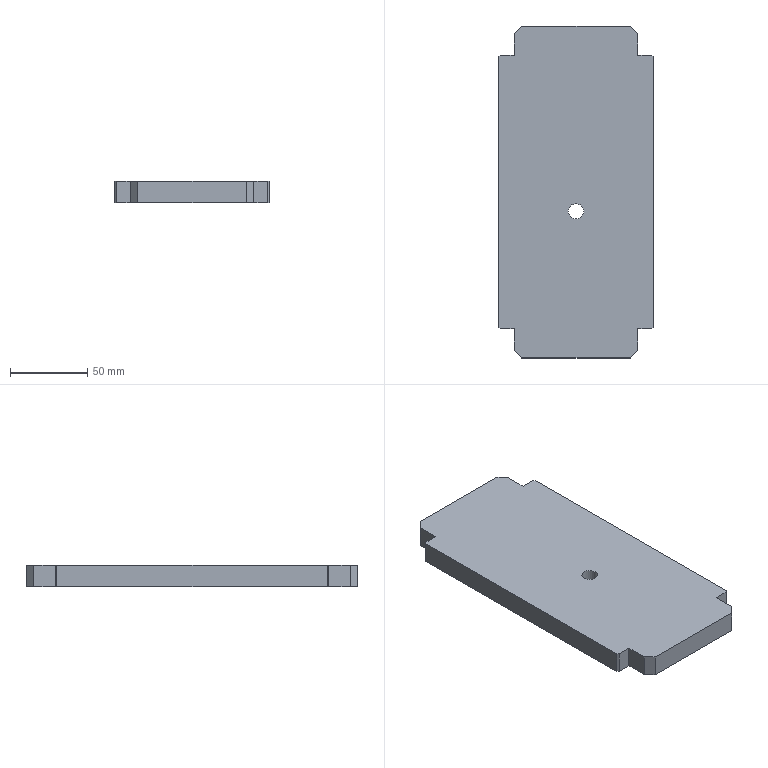Part | NX | features solid 2 | 1 solid | 23 faces | box 100 x 215 x 14 mm | volume 288532 mm3 | plane 22 | cylinder 1 | commonest cylinder face diameters 10 x1
STEP:
#1=CARTESIAN_POINT('',(-25.,296.,-5.));
#2=VERTEX_POINT('',#1);
#3=CARTESIAN_POINT('',(-34.,296.,-5.));
#4=VERTEX_POINT('',#3);
#5=CARTESIAN_POINT('',(300.,296.,-5.));
#6=DIRECTION('',(-1.,0.,0.));
#7=VECTOR('',#6,1000.);
#8=LINE('',#5,#7);
#9=EDGE_CURVE('',#2,#4,#8,.T.);
#10=ORIENTED_EDGE('',*,*,#9,.F.);
#11=CARTESIAN_POINT('',(-25.,296.,-19.));
#12=VERTEX_POINT('',#11);
#13=CARTESIAN_POINT('',(-25.,296.,-21.));
#14=DIRECTION('',(0.,0.,-1.));
#15=VECTOR('',#14,1000.);
#16=LINE('',#13,#15);
#17=EDGE_CURVE('',#2,#12,#16,.T.);
#18=ORIENTED_EDGE('',*,*,#17,.T.);
#19=CARTESIAN_POINT('',(-34.,296.,-19.));
#20=VERTEX_POINT('',#19);
#21=CARTESIAN_POINT('',(15.,296.,-19.));
#22=DIRECTION('',(-1.,0.,0.));
#23=VECTOR('',#22,1000.);
#24=LINE('',#21,#23);
#25=EDGE_CURVE('',#12,#20,#24,.T.);
#26=ORIENTED_EDGE('',*,*,#25,.T.);
#27=CARTESIAN_POINT('',(-34.,296.,-21.));
#28=DIRECTION('',(0.,0.,1.));
#29=VECTOR('',#28,1000.);
#30=LINE('',#27,#29);
#31=EDGE_CURVE('',#20,#4,#30,.T.);
#32=ORIENTED_EDGE('',*,*,#31,.T.);
#33=EDGE_LOOP('',(#10,#18,#26,#32));
#34=FACE_BOUND('',#33,.T.);
#35=CARTESIAN_POINT('',(300.,296.,-21.));
#36=DIRECTION('',(0.,1.,0.));
#37=DIRECTION('',(0.,0.,1.));
#38=AXIS2_PLACEMENT_3D('',#35,#36,#37);
#39=PLANE('',#38);
#40=ADVANCED_FACE('',(#34),#39,.T.);
#41=CARTESIAN_POINT('',(-34.,119.,-19.));
#42=VERTEX_POINT('',#41);
#43=CARTESIAN_POINT('',(-25.,119.,-19.));
#44=VERTEX_POINT('',#43);
#45=CARTESIAN_POINT('',(15.,119.,-19.));
#46=DIRECTION('',(1.,0.,0.));
#47=VECTOR('',#46,1000.);
#48=LINE('',#45,#47);
#49=EDGE_CURVE('',#42,#44,#48,.T.);
#50=ORIENTED_EDGE('',*,*,#49,.T.);
#51=CARTESIAN_POINT('',(-25.,119.,-5.));
#52=VERTEX_POINT('',#51);
#53=CARTESIAN_POINT('',(-25.,119.,-21.));
#54=DIRECTION('',(0.,0.,1.));
#55=VECTOR('',#54,1000.);
#56=LINE('',#53,#55);
#57=EDGE_CURVE('',#44,#52,#56,.T.);
#58=ORIENTED_EDGE('',*,*,#57,.T.);
#59=CARTESIAN_POINT('',(-34.,119.,-5.));
#60=VERTEX_POINT('',#59);
#61=CARTESIAN_POINT('',(-285.,119.,-5.));
#62=DIRECTION('',(1.,0.,0.));
#63=VECTOR('',#62,1000.);
#64=LINE('',#61,#63);
#65=EDGE_CURVE('',#60,#52,#64,.T.);
#66=ORIENTED_EDGE('',*,*,#65,.F.);
#67=CARTESIAN_POINT('',(-34.,119.,-21.));
#68=DIRECTION('',(0.,0.,1.));
#69=VECTOR('',#68,1000.);
#70=LINE('',#67,#69);
#71=EDGE_CURVE('',#42,#60,#70,.T.);
#72=ORIENTED_EDGE('',*,*,#71,.F.);
#73=EDGE_LOOP('',(#50,#58,#66,#72));
#74=FACE_BOUND('',#73,.T.);
#75=CARTESIAN_POINT('',(-285.,119.,-21.));
#76=DIRECTION('',(0.,-1.,0.));
#77=DIRECTION('',(1.,0.,0.));
#78=AXIS2_PLACEMENT_3D('',#75,#76,#77);
#79=PLANE('',#78);
#80=ADVANCED_FACE('',(#74),#79,.T.);
#81=CARTESIAN_POINT('',(55.,296.,-5.));
#82=VERTEX_POINT('',#81);
#83=CARTESIAN_POINT('',(55.,296.,-19.));
#84=VERTEX_POINT('',#83);
#85=CARTESIAN_POINT('',(55.,296.,-21.));
#86=DIRECTION('',(0.,0.,-1.));
#87=VECTOR('',#86,1000.);
#88=LINE('',#85,#87);
#89=EDGE_CURVE('',#82,#84,#88,.T.);
#90=ORIENTED_EDGE('',*,*,#89,.F.);
#91=CARTESIAN_POINT('',(64.,296.,-5.));
#92=VERTEX_POINT('',#91);
#93=CARTESIAN_POINT('',(300.,296.,-5.));
#94=DIRECTION('',(-1.,0.,0.));
#95=VECTOR('',#94,1000.);
#96=LINE('',#93,#95);
#97=EDGE_CURVE('',#92,#82,#96,.T.);
#98=ORIENTED_EDGE('',*,*,#97,.F.);
#99=CARTESIAN_POINT('',(64.,296.,-19.));
#100=VERTEX_POINT('',#99);
#101=CARTESIAN_POINT('',(64.,296.,-21.));
#102=DIRECTION('',(0.,0.,1.));
#103=VECTOR('',#102,1000.);
#104=LINE('',#101,#103);
#105=EDGE_CURVE('',#100,#92,#104,.T.);
#106=ORIENTED_EDGE('',*,*,#105,.F.);
#107=CARTESIAN_POINT('',(15.,296.,-19.));
#108=DIRECTION('',(-1.,0.,0.));
#109=VECTOR('',#108,1000.);
#110=LINE('',#107,#109);
#111=EDGE_CURVE('',#100,#84,#110,.T.);
#112=ORIENTED_EDGE('',*,*,#111,.T.);
#113=EDGE_LOOP('',(#90,#98,#106,#112));
#114=FACE_BOUND('',#113,.T.);
#115=CARTESIAN_POINT('',(300.,296.,-21.));
#116=DIRECTION('',(0.,1.,0.));
#117=DIRECTION('',(0.,0.,1.));
#118=AXIS2_PLACEMENT_3D('',#115,#116,#117);
#119=PLANE('',#118);
#120=ADVANCED_FACE('',(#114),#119,.T.);
#121=CARTESIAN_POINT('',(-35.,295.,-5.));
#122=VERTEX_POINT('',#121);
#123=CARTESIAN_POINT('',(-34.,296.,-5.));
#124=DIRECTION('',(-0.7071,-0.7071,0.));
#125=VECTOR('',#124,1000.);
#126=LINE('',#123,#125);
#127=EDGE_CURVE('',#4,#122,#126,.T.);
#128=ORIENTED_EDGE('',*,*,#127,.F.);
#129=ORIENTED_EDGE('',*,*,#31,.F.);
#130=CARTESIAN_POINT('',(-35.,295.,-19.));
#131=VERTEX_POINT('',#130);
#132=CARTESIAN_POINT('',(-60.,270.,-19.));
#133=DIRECTION('',(-0.7071,-0.7071,0.));
#134=VECTOR('',#133,1000.);
#135=LINE('',#132,#134);
#136=EDGE_CURVE('',#20,#131,#135,.T.);
#137=ORIENTED_EDGE('',*,*,#136,.T.);
#138=CARTESIAN_POINT('',(-35.,295.,-21.));
#139=DIRECTION('',(0.,0.,1.));
#140=VECTOR('',#139,1000.);
#141=LINE('',#138,#140);
#142=EDGE_CURVE('',#131,#122,#141,.T.);
#143=ORIENTED_EDGE('',*,*,#142,.T.);
#144=EDGE_LOOP('',(#128,#129,#137,#143));
#145=FACE_BOUND('',#144,.T.);
#146=CARTESIAN_POINT('',(-34.,296.,-21.));
#147=DIRECTION('',(-0.7071,0.7071,0.));
#148=DIRECTION('',(-0.7071,-0.7071,0.));
#149=AXIS2_PLACEMENT_3D('',#146,#147,#148);
#150=PLANE('',#149);
#151=ADVANCED_FACE('',(#145),#150,.T.);
#152=CARTESIAN_POINT('',(-35.,120.,-5.));
#153=VERTEX_POINT('',#152);
#154=CARTESIAN_POINT('',(-35.,195.,-5.));
#155=DIRECTION('',(0.,1.,0.));
#156=VECTOR('',#155,1000.);
#157=LINE('',#154,#156);
#158=EDGE_CURVE('',#153,#122,#157,.T.);
#159=ORIENTED_EDGE('',*,*,#158,.T.);
#160=ORIENTED_EDGE('',*,*,#142,.F.);
#161=CARTESIAN_POINT('',(-35.,120.,-19.));
#162=VERTEX_POINT('',#161);
#163=CARTESIAN_POINT('',(-35.,195.,-19.));
#164=DIRECTION('',(0.,1.,0.));
#165=VECTOR('',#164,1000.);
#166=LINE('',#163,#165);
#167=EDGE_CURVE('',#162,#131,#166,.T.);
#168=ORIENTED_EDGE('',*,*,#167,.F.);
#169=CARTESIAN_POINT('',(-35.,120.,-21.));
#170=DIRECTION('',(0.,0.,1.));
#171=VECTOR('',#170,1000.);
#172=LINE('',#169,#171);
#173=EDGE_CURVE('',#162,#153,#172,.T.);
#174=ORIENTED_EDGE('',*,*,#173,.T.);
#175=EDGE_LOOP('',(#159,#160,#168,#174));
#176=FACE_BOUND('',#175,.T.);
#177=CARTESIAN_POINT('',(-35.,195.,-21.));
#178=DIRECTION('',(1.,0.,0.));
#179=DIRECTION('',(0.,1.,0.));
#180=AXIS2_PLACEMENT_3D('',#177,#178,#179);
#181=PLANE('',#180);
#182=ADVANCED_FACE('',(#176),#181,.F.);
#183=CARTESIAN_POINT('',(-35.,120.,-5.));
#184=DIRECTION('',(0.7071,-0.7071,0.));
#185=VECTOR('',#184,1000.);
#186=LINE('',#183,#185);
#187=EDGE_CURVE('',#153,#60,#186,.T.);
#188=ORIENTED_EDGE('',*,*,#187,.F.);
#189=ORIENTED_EDGE('',*,*,#173,.F.);
#190=CARTESIAN_POINT('',(-47.5,132.5,-19.));
#191=DIRECTION('',(0.7071,-0.7071,0.));
#192=VECTOR('',#191,1000.);
#193=LINE('',#190,#192);
#194=EDGE_CURVE('',#162,#42,#193,.T.);
#195=ORIENTED_EDGE('',*,*,#194,.T.);
#196=ORIENTED_EDGE('',*,*,#71,.T.);
#197=EDGE_LOOP('',(#188,#189,#195,#196));
#198=FACE_BOUND('',#197,.T.);
#199=CARTESIAN_POINT('',(-35.,120.,-21.));
#200=DIRECTION('',(-0.7071,-0.7071,0.));
#201=DIRECTION('',(0.7071,-0.7071,0.));
#202=AXIS2_PLACEMENT_3D('',#199,#200,#201);
#203=PLANE('',#202);
#204=ADVANCED_FACE('',(#198),#203,.T.);
#205=CARTESIAN_POINT('',(55.,119.,-19.));
#206=VERTEX_POINT('',#205);
#207=CARTESIAN_POINT('',(55.,119.,-5.));
#208=VERTEX_POINT('',#207);
#209=CARTESIAN_POINT('',(55.,119.,-21.));
#210=DIRECTION('',(0.,0.,1.));
#211=VECTOR('',#210,1000.);
#212=LINE('',#209,#211);
#213=EDGE_CURVE('',#206,#208,#212,.T.);
#214=ORIENTED_EDGE('',*,*,#213,.F.);
#215=CARTESIAN_POINT('',(64.,119.,-19.));
#216=VERTEX_POINT('',#215);
#217=CARTESIAN_POINT('',(15.,119.,-19.));
#218=DIRECTION('',(1.,0.,0.));
#219=VECTOR('',#218,1000.);
#220=LINE('',#217,#219);
#221=EDGE_CURVE('',#206,#216,#220,.T.);
#222=ORIENTED_EDGE('',*,*,#221,.T.);
#223=CARTESIAN_POINT('',(64.,119.,-5.));
#224=VERTEX_POINT('',#223);
#225=CARTESIAN_POINT('',(64.,119.,-21.));
#226=DIRECTION('',(0.,0.,1.));
#227=VECTOR('',#226,1000.);
#228=LINE('',#225,#227);
#229=EDGE_CURVE('',#216,#224,#228,.T.);
#230=ORIENTED_EDGE('',*,*,#229,.T.);
#231=CARTESIAN_POINT('',(-285.,119.,-5.));
#232=DIRECTION('',(1.,0.,0.));
#233=VECTOR('',#232,1000.);
#234=LINE('',#231,#233);
#235=EDGE_CURVE('',#208,#224,#234,.T.);
#236=ORIENTED_EDGE('',*,*,#235,.F.);
#237=EDGE_LOOP('',(#214,#222,#230,#236));
#238=FACE_BOUND('',#237,.T.);
#239=CARTESIAN_POINT('',(-285.,119.,-21.));
#240=DIRECTION('',(0.,-1.,0.));
#241=DIRECTION('',(1.,0.,0.));
#242=AXIS2_PLACEMENT_3D('',#239,#240,#241);
#243=PLANE('',#242);
#244=ADVANCED_FACE('',(#238),#243,.T.);
#245=CARTESIAN_POINT('',(65.,120.,-5.));
#246=VERTEX_POINT('',#245);
#247=CARTESIAN_POINT('',(64.,119.,-5.));
#248=DIRECTION('',(0.7071,0.7071,0.));
#249=VECTOR('',#248,1000.);
#250=LINE('',#247,#249);
#251=EDGE_CURVE('',#224,#246,#250,.T.);
#252=ORIENTED_EDGE('',*,*,#251,.F.);
#253=ORIENTED_EDGE('',*,*,#229,.F.);
#254=CARTESIAN_POINT('',(65.,120.,-19.));
#255=VERTEX_POINT('',#254);
#256=CARTESIAN_POINT('',(77.5,132.5,-19.));
#257=DIRECTION('',(0.7071,0.7071,0.));
#258=VECTOR('',#257,1000.);
#259=LINE('',#256,#258);
#260=EDGE_CURVE('',#216,#255,#259,.T.);
#261=ORIENTED_EDGE('',*,*,#260,.T.);
#262=CARTESIAN_POINT('',(65.,120.,-21.));
#263=DIRECTION('',(0.,0.,1.));
#264=VECTOR('',#263,1000.);
#265=LINE('',#262,#264);
#266=EDGE_CURVE('',#255,#246,#265,.T.);
#267=ORIENTED_EDGE('',*,*,#266,.T.);
#268=EDGE_LOOP('',(#252,#253,#261,#267));
#269=FACE_BOUND('',#268,.T.);
#270=CARTESIAN_POINT('',(64.,119.,-21.));
#271=DIRECTION('',(0.7071,-0.7071,0.));
#272=DIRECTION('',(0.7071,0.7071,0.));
#273=AXIS2_PLACEMENT_3D('',#270,#271,#272);
#274=PLANE('',#273);
#275=ADVANCED_FACE('',(#269),#274,.T.);
#276=CARTESIAN_POINT('',(65.,295.,-5.));
#277=VERTEX_POINT('',#276);
#278=CARTESIAN_POINT('',(65.,120.,-5.));
#279=DIRECTION('',(0.,1.,0.));
#280=VECTOR('',#279,1000.);
#281=LINE('',#278,#280);
#282=EDGE_CURVE('',#246,#277,#281,.T.);
#283=ORIENTED_EDGE('',*,*,#282,.F.);
#284=ORIENTED_EDGE('',*,*,#266,.F.);
#285=CARTESIAN_POINT('',(65.,295.,-19.));
#286=VERTEX_POINT('',#285);
#287=CARTESIAN_POINT('',(65.,195.,-19.));
#288=DIRECTION('',(0.,1.,0.));
#289=VECTOR('',#288,1000.);
#290=LINE('',#287,#289);
#291=EDGE_CURVE('',#255,#286,#290,.T.);
#292=ORIENTED_EDGE('',*,*,#291,.T.);
#293=CARTESIAN_POINT('',(65.,295.,-21.));
#294=DIRECTION('',(0.,0.,1.));
#295=VECTOR('',#294,1000.);
#296=LINE('',#293,#295);
#297=EDGE_CURVE('',#286,#277,#296,.T.);
#298=ORIENTED_EDGE('',*,*,#297,.T.);
#299=EDGE_LOOP('',(#283,#284,#292,#298));
#300=FACE_BOUND('',#299,.T.);
#301=CARTESIAN_POINT('',(65.,120.,-21.));
#302=DIRECTION('',(1.,0.,0.));
#303=DIRECTION('',(0.,1.,0.));
#304=AXIS2_PLACEMENT_3D('',#301,#302,#303);
#305=PLANE('',#304);
#306=ADVANCED_FACE('',(#300),#305,.T.);
#307=CARTESIAN_POINT('',(64.,296.,-5.));
#308=DIRECTION('',(0.7071,-0.7071,0.));
#309=VECTOR('',#308,1000.);
#310=LINE('',#307,#309);
#311=EDGE_CURVE('',#92,#277,#310,.T.);
#312=ORIENTED_EDGE('',*,*,#311,.T.);
#313=ORIENTED_EDGE('',*,*,#297,.F.);
#314=CARTESIAN_POINT('',(90.,270.,-19.));
#315=DIRECTION('',(0.7071,-0.7071,0.));
#316=VECTOR('',#315,1000.);
#317=LINE('',#314,#316);
#318=EDGE_CURVE('',#100,#286,#317,.T.);
#319=ORIENTED_EDGE('',*,*,#318,.F.);
#320=ORIENTED_EDGE('',*,*,#105,.T.);
#321=EDGE_LOOP('',(#312,#313,#319,#320));
#322=FACE_BOUND('',#321,.T.);
#323=CARTESIAN_POINT('',(64.,296.,-21.));
#324=DIRECTION('',(-0.7071,-0.7071,0.));
#325=DIRECTION('',(0.7071,-0.7071,0.));
#326=AXIS2_PLACEMENT_3D('',#323,#324,#325);
#327=PLANE('',#326);
#328=ADVANCED_FACE('',(#322),#327,.F.);
#329=CARTESIAN_POINT('',(20.,195.,-19.));
#330=VERTEX_POINT('',#329);
#331=CARTESIAN_POINT('',(15.,195.,-19.));
#332=DIRECTION('',(0.,0.,1.));
#333=DIRECTION('',(1.,0.,0.));
#334=AXIS2_PLACEMENT_3D('',#331,#332,#333);
#335=CIRCLE('',#334,5.);
#336=EDGE_CURVE('',#330,#330,#335,.T.);
#337=ORIENTED_EDGE('',*,*,#336,.T.);
#338=EDGE_LOOP('',(#337));
#339=FACE_BOUND('',#338,.T.);
#340=ORIENTED_EDGE('',*,*,#221,.F.);
#341=CARTESIAN_POINT('',(55.,105.,-19.));
#342=VERTEX_POINT('',#341);
#343=CARTESIAN_POINT('',(55.,195.,-19.));
#344=DIRECTION('',(0.,1.,0.));
#345=VECTOR('',#344,1000.);
#346=LINE('',#343,#345);
#347=EDGE_CURVE('',#342,#206,#346,.T.);
#348=ORIENTED_EDGE('',*,*,#347,.F.);
#349=CARTESIAN_POINT('',(50.,100.,-19.));
#350=VERTEX_POINT('',#349);
#351=CARTESIAN_POINT('',(80.,130.,-19.));
#352=DIRECTION('',(-0.7071,-0.7071,0.));
#353=VECTOR('',#352,1000.);
#354=LINE('',#351,#353);
#355=EDGE_CURVE('',#342,#350,#354,.T.);
#356=ORIENTED_EDGE('',*,*,#355,.T.);
#357=CARTESIAN_POINT('',(-20.,100.,-19.));
#358=VERTEX_POINT('',#357);
#359=CARTESIAN_POINT('',(15.,100.,-19.));
#360=DIRECTION('',(-1.,0.,0.));
#361=VECTOR('',#360,1000.);
#362=LINE('',#359,#361);
#363=EDGE_CURVE('',#350,#358,#362,.T.);
#364=ORIENTED_EDGE('',*,*,#363,.T.);
#365=CARTESIAN_POINT('',(-25.,105.,-19.));
#366=VERTEX_POINT('',#365);
#367=CARTESIAN_POINT('',(-50.,130.,-19.));
#368=DIRECTION('',(-0.7071,0.7071,0.));
#369=VECTOR('',#368,1000.);
#370=LINE('',#367,#369);
#371=EDGE_CURVE('',#358,#366,#370,.T.);
#372=ORIENTED_EDGE('',*,*,#371,.T.);
#373=CARTESIAN_POINT('',(-25.,195.,-19.));
#374=DIRECTION('',(0.,1.,0.));
#375=VECTOR('',#374,1000.);
#376=LINE('',#373,#375);
#377=EDGE_CURVE('',#366,#44,#376,.T.);
#378=ORIENTED_EDGE('',*,*,#377,.T.);
#379=ORIENTED_EDGE('',*,*,#49,.F.);
#380=ORIENTED_EDGE('',*,*,#194,.F.);
#381=ORIENTED_EDGE('',*,*,#167,.T.);
#382=ORIENTED_EDGE('',*,*,#136,.F.);
#383=ORIENTED_EDGE('',*,*,#25,.F.);
#384=CARTESIAN_POINT('',(-25.,310.,-19.));
#385=VERTEX_POINT('',#384);
#386=CARTESIAN_POINT('',(-25.,195.,-19.));
#387=DIRECTION('',(0.,1.,0.));
#388=VECTOR('',#387,1000.);
#389=LINE('',#386,#388);
#390=EDGE_CURVE('',#12,#385,#389,.T.);
#391=ORIENTED_EDGE('',*,*,#390,.T.);
#392=CARTESIAN_POINT('',(-20.,315.,-19.));
#393=VERTEX_POINT('',#392);
#394=CARTESIAN_POINT('',(-62.5,272.5,-19.));
#395=DIRECTION('',(-0.7071,-0.7071,0.));
#396=VECTOR('',#395,1000.);
#397=LINE('',#394,#396);
#398=EDGE_CURVE('',#393,#385,#397,.T.);
#399=ORIENTED_EDGE('',*,*,#398,.F.);
#400=CARTESIAN_POINT('',(50.,315.,-19.));
#401=VERTEX_POINT('',#400);
#402=CARTESIAN_POINT('',(15.,315.,-19.));
#403=DIRECTION('',(-1.,0.,0.));
#404=VECTOR('',#403,1000.);
#405=LINE('',#402,#404);
#406=EDGE_CURVE('',#401,#393,#405,.T.);
#407=ORIENTED_EDGE('',*,*,#406,.F.);
#408=CARTESIAN_POINT('',(55.,310.,-19.));
#409=VERTEX_POINT('',#408);
#410=CARTESIAN_POINT('',(92.5,272.5,-19.));
#411=DIRECTION('',(-0.7071,0.7071,0.));
#412=VECTOR('',#411,1000.);
#413=LINE('',#410,#412);
#414=EDGE_CURVE('',#409,#401,#413,.T.);
#415=ORIENTED_EDGE('',*,*,#414,.F.);
#416=CARTESIAN_POINT('',(55.,195.,-19.));
#417=DIRECTION('',(0.,1.,0.));
#418=VECTOR('',#417,1000.);
#419=LINE('',#416,#418);
#420=EDGE_CURVE('',#84,#409,#419,.T.);
#421=ORIENTED_EDGE('',*,*,#420,.F.);
#422=ORIENTED_EDGE('',*,*,#111,.F.);
#423=ORIENTED_EDGE('',*,*,#318,.T.);
#424=ORIENTED_EDGE('',*,*,#291,.F.);
#425=ORIENTED_EDGE('',*,*,#260,.F.);
#426=EDGE_LOOP('',(#340,#348,#356,#364,#372,#378,#379,#380,#381,#382,#383,#391,#399,#407,#415,#421,#422,#423,#424,#425));
#427=FACE_BOUND('',#426,.T.);
#428=CARTESIAN_POINT('',(15.,195.,-19.));
#429=DIRECTION('',(0.,0.,1.));
#430=DIRECTION('',(1.,0.,0.));
#431=AXIS2_PLACEMENT_3D('',#428,#429,#430);
#432=PLANE('',#431);
#433=ADVANCED_FACE('',(#339,#427),#432,.F.);
#434=CARTESIAN_POINT('',(20.,195.,-5.));
#435=VERTEX_POINT('',#434);
#436=CARTESIAN_POINT('',(15.,195.,-5.));
#437=DIRECTION('',(0.,0.,1.));
#438=DIRECTION('',(1.,0.,0.));
#439=AXIS2_PLACEMENT_3D('',#436,#437,#438);
#440=CIRCLE('',#439,5.);
#441=EDGE_CURVE('',#435,#435,#440,.T.);
#442=ORIENTED_EDGE('',*,*,#441,.F.);
#443=EDGE_LOOP('',(#442));
#444=FACE_BOUND('',#443,.T.);
#445=ORIENTED_EDGE('',*,*,#97,.T.);
#446=CARTESIAN_POINT('',(55.,310.,-5.));
#447=VERTEX_POINT('',#446);
#448=CARTESIAN_POINT('',(55.,105.,-5.));
#449=DIRECTION('',(0.,1.,0.));
#450=VECTOR('',#449,1000.);
#451=LINE('',#448,#450);
#452=EDGE_CURVE('',#82,#447,#451,.T.);
#453=ORIENTED_EDGE('',*,*,#452,.T.);
#454=CARTESIAN_POINT('',(50.,315.,-5.));
#455=VERTEX_POINT('',#454);
#456=CARTESIAN_POINT('',(55.,310.,-5.));
#457=DIRECTION('',(-0.7071,0.7071,0.));
#458=VECTOR('',#457,1000.);
#459=LINE('',#456,#458);
#460=EDGE_CURVE('',#447,#455,#459,.T.);
#461=ORIENTED_EDGE('',*,*,#460,.T.);
#462=CARTESIAN_POINT('',(-20.,315.,-5.));
#463=VERTEX_POINT('',#462);
#464=CARTESIAN_POINT('',(50.,315.,-5.));
#465=DIRECTION('',(-1.,0.,0.));
#466=VECTOR('',#465,1000.);
#467=LINE('',#464,#466);
#468=EDGE_CURVE('',#455,#463,#467,.T.);
#469=ORIENTED_EDGE('',*,*,#468,.T.);
#470=CARTESIAN_POINT('',(-25.,310.,-5.));
#471=VERTEX_POINT('',#470);
#472=CARTESIAN_POINT('',(-20.,315.,-5.));
#473=DIRECTION('',(-0.7071,-0.7071,0.));
#474=VECTOR('',#473,1000.);
#475=LINE('',#472,#474);
#476=EDGE_CURVE('',#463,#471,#475,.T.);
#477=ORIENTED_EDGE('',*,*,#476,.T.);
#478=CARTESIAN_POINT('',(-25.,296.,-5.));
#479=DIRECTION('',(0.,1.,0.));
#480=VECTOR('',#479,1000.);
#481=LINE('',#478,#480);
#482=EDGE_CURVE('',#2,#471,#481,.T.);
#483=ORIENTED_EDGE('',*,*,#482,.F.);
#484=ORIENTED_EDGE('',*,*,#9,.T.);
#485=ORIENTED_EDGE('',*,*,#127,.T.);
#486=ORIENTED_EDGE('',*,*,#158,.F.);
#487=ORIENTED_EDGE('',*,*,#187,.T.);
#488=ORIENTED_EDGE('',*,*,#65,.T.);
#489=CARTESIAN_POINT('',(-25.,105.,-5.));
#490=VERTEX_POINT('',#489);
#491=CARTESIAN_POINT('',(-25.,296.,-5.));
#492=DIRECTION('',(0.,1.,0.));
#493=VECTOR('',#492,1000.);
#494=LINE('',#491,#493);
#495=EDGE_CURVE('',#490,#52,#494,.T.);
#496=ORIENTED_EDGE('',*,*,#495,.F.);
#497=CARTESIAN_POINT('',(-20.,100.,-5.));
#498=VERTEX_POINT('',#497);
#499=CARTESIAN_POINT('',(-20.,100.,-5.));
#500=DIRECTION('',(-0.7071,0.7071,0.));
#501=VECTOR('',#500,1000.);
#502=LINE('',#499,#501);
#503=EDGE_CURVE('',#498,#490,#502,.T.);
#504=ORIENTED_EDGE('',*,*,#503,.F.);
#505=CARTESIAN_POINT('',(50.,100.,-5.));
#506=VERTEX_POINT('',#505);
#507=CARTESIAN_POINT('',(50.,100.,-5.));
#508=DIRECTION('',(-1.,0.,0.));
#509=VECTOR('',#508,1000.);
#510=LINE('',#507,#509);
#511=EDGE_CURVE('',#506,#498,#510,.T.);
#512=ORIENTED_EDGE('',*,*,#511,.F.);
#513=CARTESIAN_POINT('',(55.,105.,-5.));
#514=VERTEX_POINT('',#513);
#515=CARTESIAN_POINT('',(55.,105.,-5.));
#516=DIRECTION('',(-0.7071,-0.7071,0.));
#517=VECTOR('',#516,1000.);
#518=LINE('',#515,#517);
#519=EDGE_CURVE('',#514,#506,#518,.T.);
#520=ORIENTED_EDGE('',*,*,#519,.F.);
#521=CARTESIAN_POINT('',(55.,105.,-5.));
#522=DIRECTION('',(0.,1.,0.));
#523=VECTOR('',#522,1000.);
#524=LINE('',#521,#523);
#525=EDGE_CURVE('',#514,#208,#524,.T.);
#526=ORIENTED_EDGE('',*,*,#525,.T.);
#527=ORIENTED_EDGE('',*,*,#235,.T.);
#528=ORIENTED_EDGE('',*,*,#251,.T.);
#529=ORIENTED_EDGE('',*,*,#282,.T.);
#530=ORIENTED_EDGE('',*,*,#311,.F.);
#531=EDGE_LOOP('',(#445,#453,#461,#469,#477,#483,#484,#485,#486,#487,#488,#496,#504,#512,#520,#526,#527,#528,#529,#530));
#532=FACE_BOUND('',#531,.T.);
#533=CARTESIAN_POINT('',(7.778,186.667,-5.));
#534=DIRECTION('',(0.,0.,1.));
#535=DIRECTION('',(1.,0.,0.));
#536=AXIS2_PLACEMENT_3D('',#533,#534,#535);
#537=PLANE('',#536);
#538=ADVANCED_FACE('',(#444,#532),#537,.T.);
#539=ORIENTED_EDGE('',*,*,#519,.T.);
#540=CARTESIAN_POINT('',(50.,100.,-21.));
#541=DIRECTION('',(0.,0.,1.));
#542=VECTOR('',#541,1000.);
#543=LINE('',#540,#542);
#544=EDGE_CURVE('',#350,#506,#543,.T.);
#545=ORIENTED_EDGE('',*,*,#544,.F.);
#546=ORIENTED_EDGE('',*,*,#355,.F.);
#547=CARTESIAN_POINT('',(55.,105.,-21.));
#548=DIRECTION('',(0.,0.,1.));
#549=VECTOR('',#548,1000.);
#550=LINE('',#547,#549);
#551=EDGE_CURVE('',#342,#514,#550,.T.);
#552=ORIENTED_EDGE('',*,*,#551,.T.);
#553=EDGE_LOOP('',(#539,#545,#546,#552));
#554=FACE_BOUND('',#553,.T.);
#555=CARTESIAN_POINT('',(55.,105.,-21.));
#556=DIRECTION('',(-0.7071,0.7071,0.));
#557=DIRECTION('',(-0.7071,-0.7071,0.));
#558=AXIS2_PLACEMENT_3D('',#555,#556,#557);
#559=PLANE('',#558);
#560=ADVANCED_FACE('',(#554),#559,.F.);
#561=ORIENTED_EDGE('',*,*,#511,.T.);
#562=CARTESIAN_POINT('',(-20.,100.,-21.));
#563=DIRECTION('',(0.,0.,1.));
#564=VECTOR('',#563,1000.);
#565=LINE('',#562,#564);
#566=EDGE_CURVE('',#358,#498,#565,.T.);
#567=ORIENTED_EDGE('',*,*,#566,.F.);
#568=ORIENTED_EDGE('',*,*,#363,.F.);
#569=ORIENTED_EDGE('',*,*,#544,.T.);
#570=EDGE_LOOP('',(#561,#567,#568,#569));
#571=FACE_BOUND('',#570,.T.);
#572=CARTESIAN_POINT('',(50.,100.,-21.));
#573=DIRECTION('',(0.,1.,0.));
#574=DIRECTION('',(0.,0.,1.));
#575=AXIS2_PLACEMENT_3D('',#572,#573,#574);
#576=PLANE('',#575);
#577=ADVANCED_FACE('',(#571),#576,.F.);
#578=ORIENTED_EDGE('',*,*,#503,.T.);
#579=CARTESIAN_POINT('',(-25.,105.,-21.));
#580=DIRECTION('',(0.,0.,1.));
#581=VECTOR('',#580,1000.);
#582=LINE('',#579,#581);
#583=EDGE_CURVE('',#366,#490,#582,.T.);
#584=ORIENTED_EDGE('',*,*,#583,.F.);
#585=ORIENTED_EDGE('',*,*,#371,.F.);
#586=ORIENTED_EDGE('',*,*,#566,.T.);
#587=EDGE_LOOP('',(#578,#584,#585,#586));
#588=FACE_BOUND('',#587,.T.);
#589=CARTESIAN_POINT('',(-20.,100.,-21.));
#590=DIRECTION('',(0.7071,0.7071,0.));
#591=DIRECTION('',(-0.7071,0.7071,0.));
#592=AXIS2_PLACEMENT_3D('',#589,#590,#591);
#593=PLANE('',#592);
#594=ADVANCED_FACE('',(#588),#593,.F.);
#595=ORIENTED_EDGE('',*,*,#347,.T.);
#596=ORIENTED_EDGE('',*,*,#213,.T.);
#597=ORIENTED_EDGE('',*,*,#525,.F.);
#598=ORIENTED_EDGE('',*,*,#551,.F.);
#599=EDGE_LOOP('',(#595,#596,#597,#598));
#600=FACE_BOUND('',#599,.T.);
#601=CARTESIAN_POINT('',(55.,105.,-21.));
#602=DIRECTION('',(1.,0.,0.));
#603=DIRECTION('',(0.,0.,-1.));
#604=AXIS2_PLACEMENT_3D('',#601,#602,#603);
#605=PLANE('',#604);
#606=ADVANCED_FACE('',(#600),#605,.T.);
#607=ORIENTED_EDGE('',*,*,#57,.F.);
#608=ORIENTED_EDGE('',*,*,#377,.F.);
#609=ORIENTED_EDGE('',*,*,#583,.T.);
#610=ORIENTED_EDGE('',*,*,#495,.T.);
#611=EDGE_LOOP('',(#607,#608,#609,#610));
#612=FACE_BOUND('',#611,.T.);
#613=CARTESIAN_POINT('',(-25.,296.,-21.));
#614=DIRECTION('',(1.,0.,0.));
#615=DIRECTION('',(0.,0.,-1.));
#616=AXIS2_PLACEMENT_3D('',#613,#614,#615);
#617=PLANE('',#616);
#618=ADVANCED_FACE('',(#612),#617,.F.);
#619=ORIENTED_EDGE('',*,*,#17,.F.);
#620=ORIENTED_EDGE('',*,*,#482,.T.);
#621=CARTESIAN_POINT('',(-25.,310.,-21.));
#622=DIRECTION('',(0.,0.,1.));
#623=VECTOR('',#622,1000.);
#624=LINE('',#621,#623);
#625=EDGE_CURVE('',#385,#471,#624,.T.);
#626=ORIENTED_EDGE('',*,*,#625,.F.);
#627=ORIENTED_EDGE('',*,*,#390,.F.);
#628=EDGE_LOOP('',(#619,#620,#626,#627));
#629=FACE_BOUND('',#628,.T.);
#630=CARTESIAN_POINT('',(-25.,296.,-21.));
#631=DIRECTION('',(1.,0.,0.));
#632=DIRECTION('',(0.,0.,-1.));
#633=AXIS2_PLACEMENT_3D('',#630,#631,#632);
#634=PLANE('',#633);
#635=ADVANCED_FACE('',(#629),#634,.F.);
#636=ORIENTED_EDGE('',*,*,#452,.F.);
#637=ORIENTED_EDGE('',*,*,#89,.T.);
#638=ORIENTED_EDGE('',*,*,#420,.T.);
#639=CARTESIAN_POINT('',(55.,310.,-21.));
#640=DIRECTION('',(0.,0.,1.));
#641=VECTOR('',#640,1000.);
#642=LINE('',#639,#641);
#643=EDGE_CURVE('',#409,#447,#642,.T.);
#644=ORIENTED_EDGE('',*,*,#643,.T.);
#645=EDGE_LOOP('',(#636,#637,#638,#644));
#646=FACE_BOUND('',#645,.T.);
#647=CARTESIAN_POINT('',(55.,105.,-21.));
#648=DIRECTION('',(1.,0.,0.));
#649=DIRECTION('',(0.,0.,-1.));
#650=AXIS2_PLACEMENT_3D('',#647,#648,#649);
#651=PLANE('',#650);
#652=ADVANCED_FACE('',(#646),#651,.T.);
#653=ORIENTED_EDGE('',*,*,#476,.F.);
#654=CARTESIAN_POINT('',(-20.,315.,-21.));
#655=DIRECTION('',(0.,0.,1.));
#656=VECTOR('',#655,1000.);
#657=LINE('',#654,#656);
#658=EDGE_CURVE('',#393,#463,#657,.T.);
#659=ORIENTED_EDGE('',*,*,#658,.F.);
#660=ORIENTED_EDGE('',*,*,#398,.T.);
#661=ORIENTED_EDGE('',*,*,#625,.T.);
#662=EDGE_LOOP('',(#653,#659,#660,#661));
#663=FACE_BOUND('',#662,.T.);
#664=CARTESIAN_POINT('',(-20.,315.,-21.));
#665=DIRECTION('',(-0.7071,0.7071,0.));
#666=DIRECTION('',(-0.7071,-0.7071,0.));
#667=AXIS2_PLACEMENT_3D('',#664,#665,#666);
#668=PLANE('',#667);
#669=ADVANCED_FACE('',(#663),#668,.T.);
#670=ORIENTED_EDGE('',*,*,#468,.F.);
#671=CARTESIAN_POINT('',(50.,315.,-21.));
#672=DIRECTION('',(0.,0.,1.));
#673=VECTOR('',#672,1000.);
#674=LINE('',#671,#673);
#675=EDGE_CURVE('',#401,#455,#674,.T.);
#676=ORIENTED_EDGE('',*,*,#675,.F.);
#677=ORIENTED_EDGE('',*,*,#406,.T.);
#678=ORIENTED_EDGE('',*,*,#658,.T.);
#679=EDGE_LOOP('',(#670,#676,#677,#678));
#680=FACE_BOUND('',#679,.T.);
#681=CARTESIAN_POINT('',(50.,315.,-21.));
#682=DIRECTION('',(0.,1.,0.));
#683=DIRECTION('',(0.,0.,1.));
#684=AXIS2_PLACEMENT_3D('',#681,#682,#683);
#685=PLANE('',#684);
#686=ADVANCED_FACE('',(#680),#685,.T.);
#687=ORIENTED_EDGE('',*,*,#460,.F.);
#688=ORIENTED_EDGE('',*,*,#643,.F.);
#689=ORIENTED_EDGE('',*,*,#414,.T.);
#690=ORIENTED_EDGE('',*,*,#675,.T.);
#691=EDGE_LOOP('',(#687,#688,#689,#690));
#692=FACE_BOUND('',#691,.T.);
#693=CARTESIAN_POINT('',(55.,310.,-21.));
#694=DIRECTION('',(0.7071,0.7071,0.));
#695=DIRECTION('',(-0.7071,0.7071,0.));
#696=AXIS2_PLACEMENT_3D('',#693,#694,#695);
#697=PLANE('',#696);
#698=ADVANCED_FACE('',(#692),#697,.T.);
#699=ORIENTED_EDGE('',*,*,#441,.T.);
#700=EDGE_LOOP('',(#699));
#701=FACE_BOUND('',#700,.T.);
#702=ORIENTED_EDGE('',*,*,#336,.F.);
#703=EDGE_LOOP('',(#702));
#704=FACE_BOUND('',#703,.T.);
#705=CARTESIAN_POINT('',(15.,195.,-505.));
#706=DIRECTION('',(0.,0.,1.));
#707=DIRECTION('',(1.,0.,0.));
#708=AXIS2_PLACEMENT_3D('',#705,#706,#707);
#709=CYLINDRICAL_SURFACE('',#708,5.);
#710=ADVANCED_FACE('',(#701,#704),#709,.F.);
#711=CLOSED_SHELL('',(#40,#80,#120,#151,#182,#204,#244,#275,#306,#328,#433,#538,#560,#577,#594,#606,#618,#635,#652,#669,#686,#698,#710));
#712=MANIFOLD_SOLID_BREP('',#711);
#713=(LENGTH_UNIT()NAMED_UNIT(*)SI_UNIT(.MILLI.,.METRE.));
#714=UNCERTAINTY_MEASURE_WITH_UNIT(LENGTH_MEASURE(0.00001),#713,'','');
#715=(NAMED_UNIT(*)PLANE_ANGLE_UNIT()SI_UNIT($,.RADIAN.));
#716=(NAMED_UNIT(*)SI_UNIT($,.STERADIAN.)SOLID_ANGLE_UNIT());
#717=(GEOMETRIC_REPRESENTATION_CONTEXT(3)GLOBAL_UNCERTAINTY_ASSIGNED_CONTEXT((#714))GLOBAL_UNIT_ASSIGNED_CONTEXT((#713,#715,#716))REPRESENTATION_CONTEXT('',''));
#718=ADVANCED_BREP_SHAPE_REPRESENTATION('',(#712),#717);